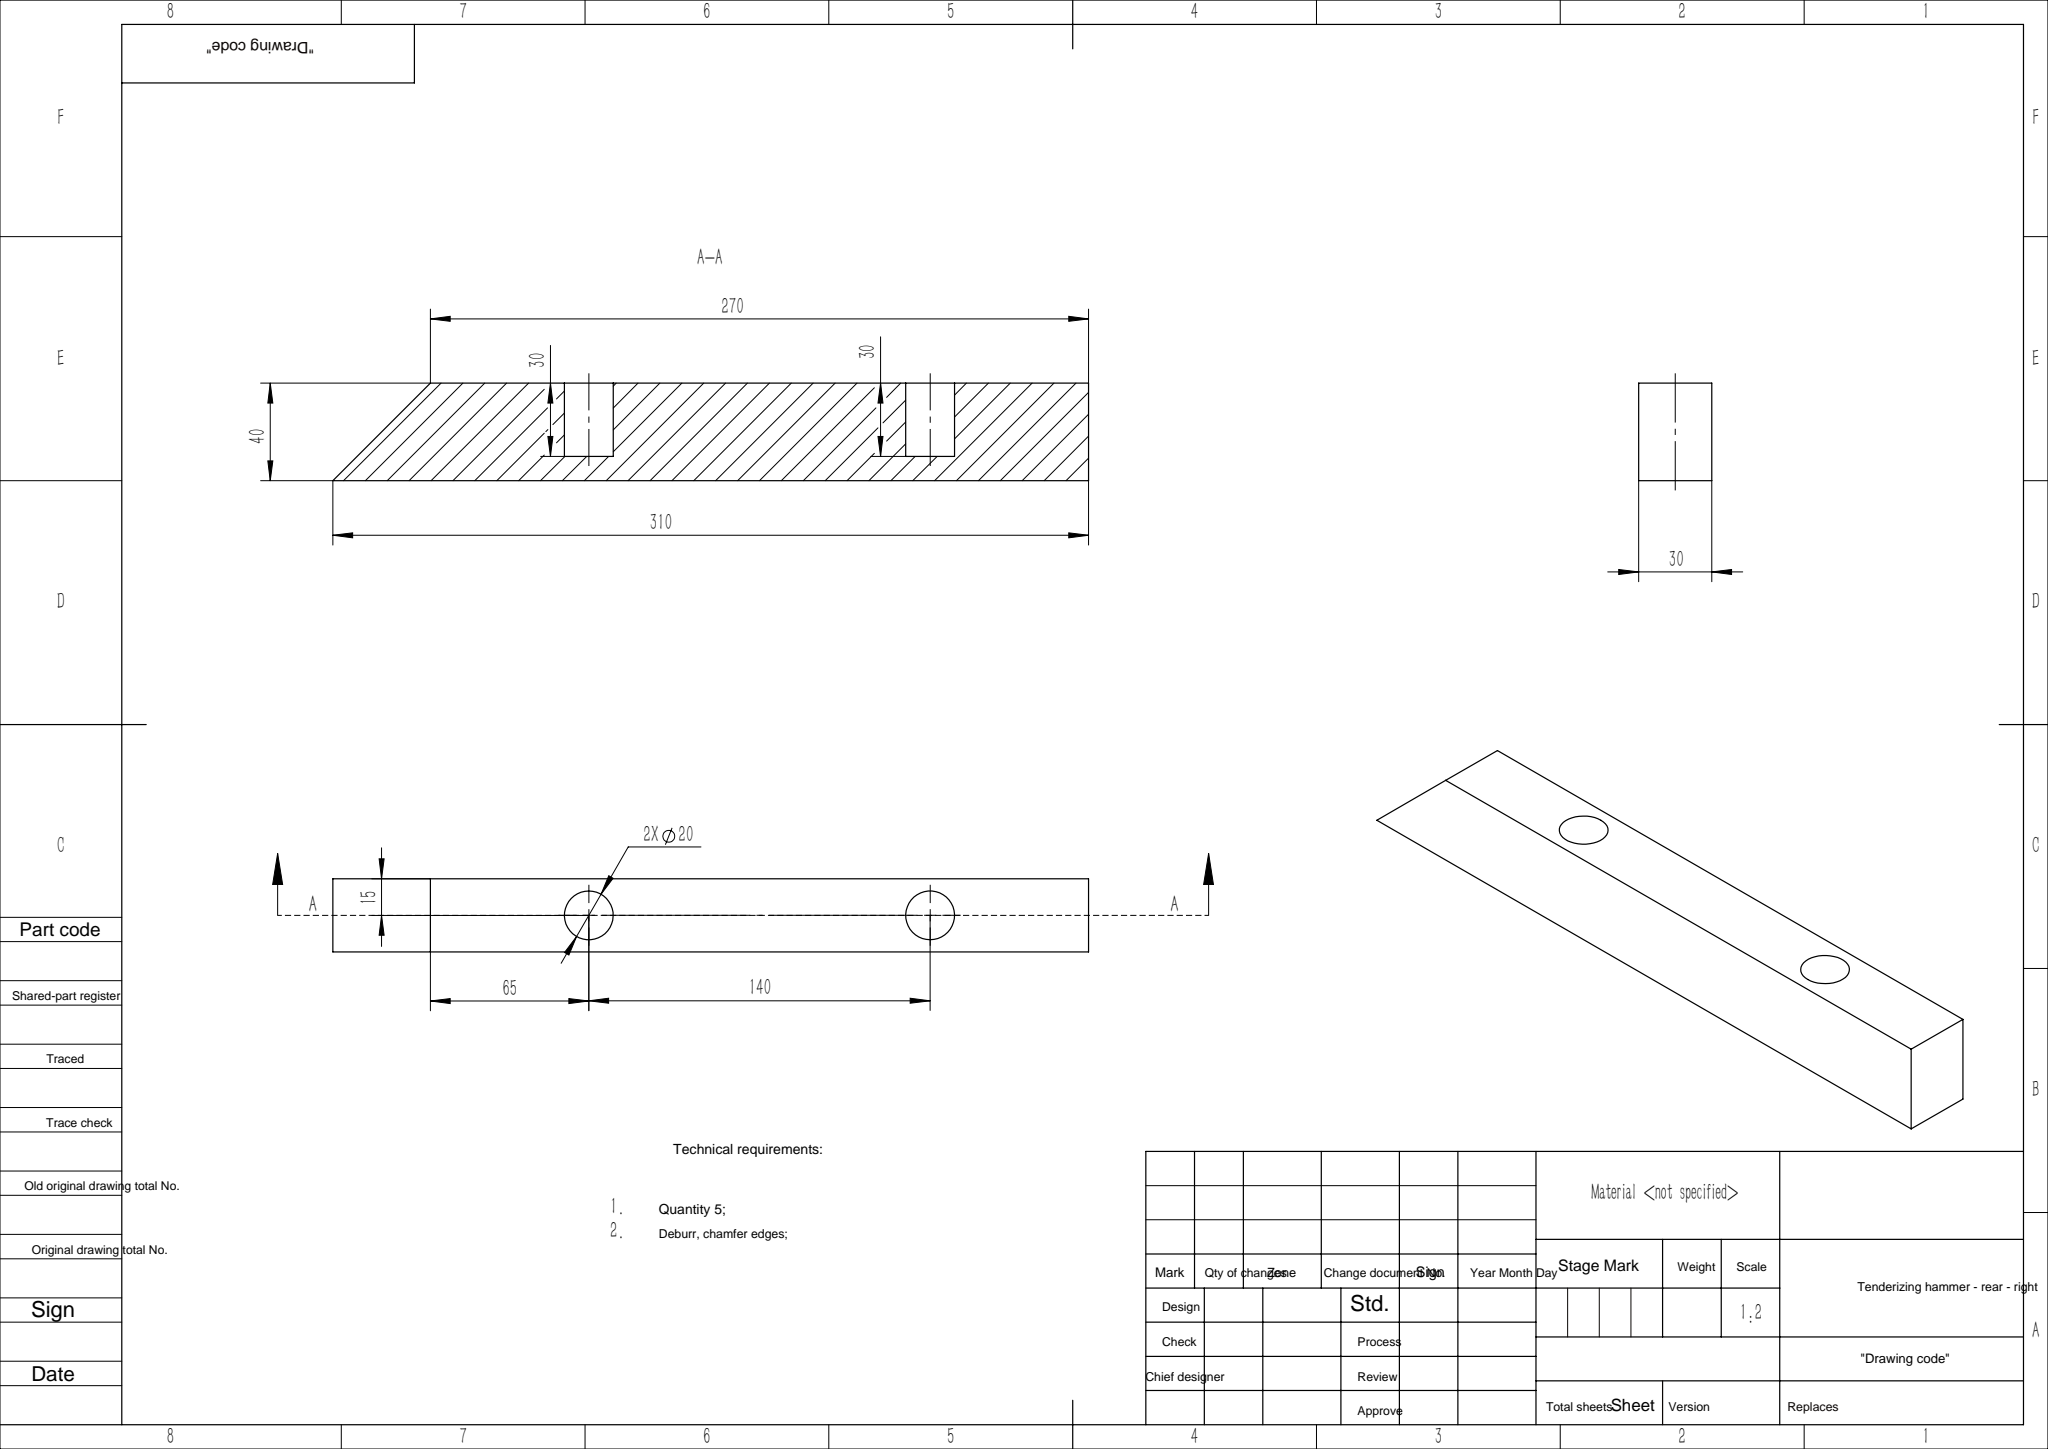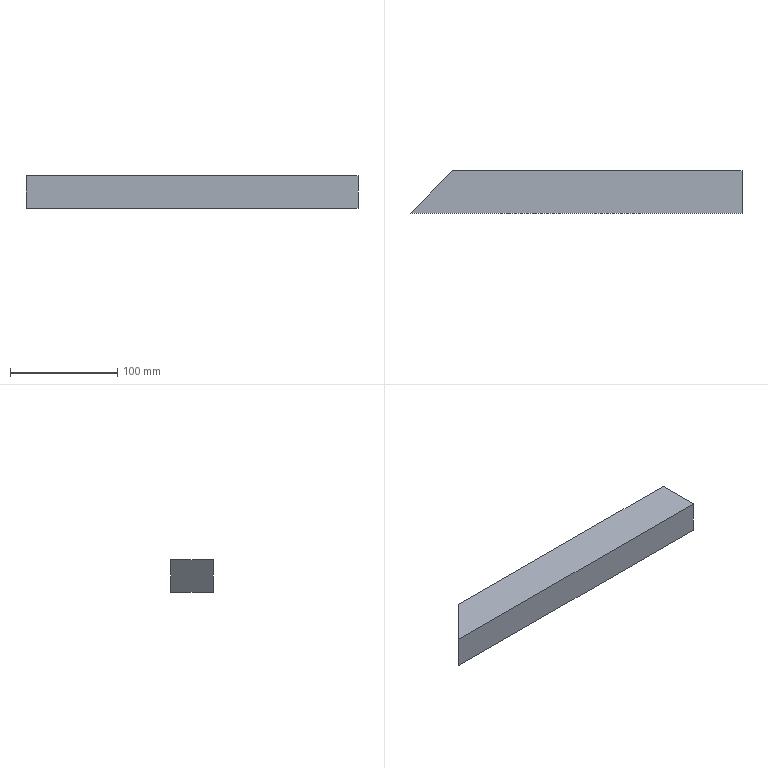Part | SolidWorks | features ICE 3, Extrusion 1 | 1 solid | 12 faces | box 310 x 40 x 30 mm | volume 329150 mm3 | plane 8 | cylinder 4 | commonest cylinder face diameters 20 x4
STEP:
#1=CARTESIAN_POINT('',(-70.,10.,-10.));
#2=VERTEX_POINT('',#1);
#3=CARTESIAN_POINT('',(-70.,10.,10.));
#4=VERTEX_POINT('',#3);
#5=CARTESIAN_POINT('',(-70.,10.,0.));
#6=DIRECTION('',(0.,1.,0.));
#7=DIRECTION('',(0.,0.,-1.));
#8=AXIS2_PLACEMENT_3D('',#5,#6,#7);
#9=CIRCLE('',#8,10.);
#10=EDGE_CURVE('',#2,#4,#9,.T.);
#11=ORIENTED_EDGE('',*,*,#10,.F.);
#12=CARTESIAN_POINT('',(-70.,40.,-10.));
#13=VERTEX_POINT('',#12);
#14=CARTESIAN_POINT('',(-70.,10.,-10.));
#15=DIRECTION('',(0.,1.,0.));
#16=VECTOR('',#15,1000.);
#17=LINE('',#14,#16);
#18=EDGE_CURVE('',#2,#13,#17,.T.);
#19=ORIENTED_EDGE('',*,*,#18,.T.);
#20=CARTESIAN_POINT('',(-70.,40.,10.));
#21=VERTEX_POINT('',#20);
#22=CARTESIAN_POINT('',(-70.,40.,0.));
#23=DIRECTION('',(0.,1.,0.));
#24=DIRECTION('',(0.,0.,-1.));
#25=AXIS2_PLACEMENT_3D('',#22,#23,#24);
#26=CIRCLE('',#25,10.);
#27=EDGE_CURVE('',#13,#21,#26,.T.);
#28=ORIENTED_EDGE('',*,*,#27,.T.);
#29=CARTESIAN_POINT('',(-70.,10.,10.));
#30=DIRECTION('',(0.,1.,0.));
#31=VECTOR('',#30,1000.);
#32=LINE('',#29,#31);
#33=EDGE_CURVE('',#4,#21,#32,.T.);
#34=ORIENTED_EDGE('',*,*,#33,.F.);
#35=EDGE_LOOP('',(#11,#19,#28,#34));
#36=FACE_OUTER_BOUND('',#35,.T.);
#37=CARTESIAN_POINT('',(-70.,10.,0.));
#38=DIRECTION('',(0.,1.,0.));
#39=DIRECTION('',(0.,0.,1.));
#40=AXIS2_PLACEMENT_3D('',#37,#38,#39);
#41=CYLINDRICAL_SURFACE('',#40,10.);
#42=ADVANCED_FACE('',(#36),#41,.F.);
#43=CARTESIAN_POINT('',(70.,10.,-10.));
#44=VERTEX_POINT('',#43);
#45=CARTESIAN_POINT('',(70.,10.,10.));
#46=VERTEX_POINT('',#45);
#47=CARTESIAN_POINT('',(70.,10.,0.));
#48=DIRECTION('',(0.,1.,0.));
#49=DIRECTION('',(0.,0.,1.));
#50=AXIS2_PLACEMENT_3D('',#47,#48,#49);
#51=CIRCLE('',#50,10.);
#52=EDGE_CURVE('',#44,#46,#51,.T.);
#53=ORIENTED_EDGE('',*,*,#52,.F.);
#54=CARTESIAN_POINT('',(70.,40.,-10.));
#55=VERTEX_POINT('',#54);
#56=CARTESIAN_POINT('',(70.,10.,-10.));
#57=DIRECTION('',(0.,1.,0.));
#58=VECTOR('',#57,1000.);
#59=LINE('',#56,#58);
#60=EDGE_CURVE('',#44,#55,#59,.T.);
#61=ORIENTED_EDGE('',*,*,#60,.T.);
#62=CARTESIAN_POINT('',(70.,40.,10.));
#63=VERTEX_POINT('',#62);
#64=CARTESIAN_POINT('',(70.,40.,0.));
#65=DIRECTION('',(0.,1.,0.));
#66=DIRECTION('',(0.,0.,1.));
#67=AXIS2_PLACEMENT_3D('',#64,#65,#66);
#68=CIRCLE('',#67,10.);
#69=EDGE_CURVE('',#55,#63,#68,.T.);
#70=ORIENTED_EDGE('',*,*,#69,.T.);
#71=CARTESIAN_POINT('',(70.,10.,10.));
#72=DIRECTION('',(0.,1.,0.));
#73=VECTOR('',#72,1000.);
#74=LINE('',#71,#73);
#75=EDGE_CURVE('',#46,#63,#74,.T.);
#76=ORIENTED_EDGE('',*,*,#75,.F.);
#77=EDGE_LOOP('',(#53,#61,#70,#76));
#78=FACE_OUTER_BOUND('',#77,.T.);
#79=CARTESIAN_POINT('',(70.,10.,0.));
#80=DIRECTION('',(0.,1.,0.));
#81=DIRECTION('',(0.,0.,1.));
#82=AXIS2_PLACEMENT_3D('',#79,#80,#81);
#83=CYLINDRICAL_SURFACE('',#82,10.);
#84=ADVANCED_FACE('',(#78),#83,.F.);
#85=CARTESIAN_POINT('',(135.,0.,15.));
#86=VERTEX_POINT('',#85);
#87=CARTESIAN_POINT('',(135.,0.,-15.));
#88=VERTEX_POINT('',#87);
#89=CARTESIAN_POINT('',(135.,0.,15.));
#90=DIRECTION('',(0.,0.,-1.));
#91=VECTOR('',#90,1000.);
#92=LINE('',#89,#91);
#93=EDGE_CURVE('',#86,#88,#92,.T.);
#94=ORIENTED_EDGE('',*,*,#93,.T.);
#95=CARTESIAN_POINT('',(135.,40.,-15.));
#96=VERTEX_POINT('',#95);
#97=CARTESIAN_POINT('',(135.,40.,-15.));
#98=DIRECTION('',(0.,-1.,0.));
#99=VECTOR('',#98,1000.);
#100=LINE('',#97,#99);
#101=EDGE_CURVE('',#96,#88,#100,.T.);
#102=ORIENTED_EDGE('',*,*,#101,.F.);
#103=CARTESIAN_POINT('',(135.,40.,15.));
#104=VERTEX_POINT('',#103);
#105=CARTESIAN_POINT('',(135.,40.,15.));
#106=DIRECTION('',(0.,0.,-1.));
#107=VECTOR('',#106,1000.);
#108=LINE('',#105,#107);
#109=EDGE_CURVE('',#104,#96,#108,.T.);
#110=ORIENTED_EDGE('',*,*,#109,.F.);
#111=CARTESIAN_POINT('',(135.,40.,15.));
#112=DIRECTION('',(0.,-1.,0.));
#113=VECTOR('',#112,1000.);
#114=LINE('',#111,#113);
#115=EDGE_CURVE('',#104,#86,#114,.T.);
#116=ORIENTED_EDGE('',*,*,#115,.T.);
#117=EDGE_LOOP('',(#94,#102,#110,#116));
#118=FACE_OUTER_BOUND('',#117,.T.);
#119=CARTESIAN_POINT('',(135.,40.,15.));
#120=DIRECTION('',(-1.,0.,0.));
#121=DIRECTION('',(0.,0.,1.));
#122=AXIS2_PLACEMENT_3D('',#119,#120,#121);
#123=PLANE('',#122);
#124=ADVANCED_FACE('',(#118),#123,.F.);
#125=CARTESIAN_POINT('',(-175.,0.,-15.));
#126=VERTEX_POINT('',#125);
#127=CARTESIAN_POINT('',(-135.,0.,-15.));
#128=DIRECTION('',(-1.,0.,0.));
#129=VECTOR('',#128,1000.);
#130=LINE('',#127,#129);
#131=EDGE_CURVE('',#88,#126,#130,.T.);
#132=ORIENTED_EDGE('',*,*,#131,.T.);
#133=CARTESIAN_POINT('',(-135.,40.,-15.));
#134=VERTEX_POINT('',#133);
#135=CARTESIAN_POINT('',(-175.,0.,-15.));
#136=DIRECTION('',(0.7071,0.7071,0.));
#137=VECTOR('',#136,1000.);
#138=LINE('',#135,#137);
#139=EDGE_CURVE('',#126,#134,#138,.T.);
#140=ORIENTED_EDGE('',*,*,#139,.T.);
#141=CARTESIAN_POINT('',(-135.,40.,-15.));
#142=DIRECTION('',(-1.,0.,0.));
#143=VECTOR('',#142,1000.);
#144=LINE('',#141,#143);
#145=EDGE_CURVE('',#96,#134,#144,.T.);
#146=ORIENTED_EDGE('',*,*,#145,.F.);
#147=ORIENTED_EDGE('',*,*,#101,.T.);
#148=EDGE_LOOP('',(#132,#140,#146,#147));
#149=FACE_OUTER_BOUND('',#148,.T.);
#150=CARTESIAN_POINT('',(-135.,40.,-15.));
#151=DIRECTION('',(0.,0.,1.));
#152=DIRECTION('',(1.,0.,0.));
#153=AXIS2_PLACEMENT_3D('',#150,#151,#152);
#154=PLANE('',#153);
#155=ADVANCED_FACE('',(#149),#154,.F.);
#156=CARTESIAN_POINT('',(-135.,40.,15.));
#157=VERTEX_POINT('',#156);
#158=CARTESIAN_POINT('',(-135.,40.,15.));
#159=DIRECTION('',(1.,0.,0.));
#160=VECTOR('',#159,1000.);
#161=LINE('',#158,#160);
#162=EDGE_CURVE('',#157,#104,#161,.T.);
#163=ORIENTED_EDGE('',*,*,#162,.F.);
#164=CARTESIAN_POINT('',(-175.,0.,15.));
#165=VERTEX_POINT('',#164);
#166=CARTESIAN_POINT('',(-175.,0.,15.));
#167=DIRECTION('',(0.7071,0.7071,0.));
#168=VECTOR('',#167,1000.);
#169=LINE('',#166,#168);
#170=EDGE_CURVE('',#165,#157,#169,.T.);
#171=ORIENTED_EDGE('',*,*,#170,.F.);
#172=CARTESIAN_POINT('',(-135.,0.,15.));
#173=DIRECTION('',(1.,0.,0.));
#174=VECTOR('',#173,1000.);
#175=LINE('',#172,#174);
#176=EDGE_CURVE('',#165,#86,#175,.T.);
#177=ORIENTED_EDGE('',*,*,#176,.T.);
#178=ORIENTED_EDGE('',*,*,#115,.F.);
#179=EDGE_LOOP('',(#163,#171,#177,#178));
#180=FACE_OUTER_BOUND('',#179,.T.);
#181=CARTESIAN_POINT('',(-135.,40.,15.));
#182=DIRECTION('',(0.,0.,-1.));
#183=DIRECTION('',(-1.,0.,0.));
#184=AXIS2_PLACEMENT_3D('',#181,#182,#183);
#185=PLANE('',#184);
#186=ADVANCED_FACE('',(#180),#185,.F.);
#187=CARTESIAN_POINT('',(-70.,40.,0.));
#188=DIRECTION('',(0.,1.,0.));
#189=DIRECTION('',(0.,0.,-1.));
#190=AXIS2_PLACEMENT_3D('',#187,#188,#189);
#191=CIRCLE('',#190,10.);
#192=EDGE_CURVE('',#21,#13,#191,.T.);
#193=ORIENTED_EDGE('',*,*,#192,.F.);
#194=ORIENTED_EDGE('',*,*,#27,.F.);
#195=EDGE_LOOP('',(#193,#194));
#196=FACE_BOUND('',#195,.T.);
#197=CARTESIAN_POINT('',(70.,40.,0.));
#198=DIRECTION('',(0.,1.,0.));
#199=DIRECTION('',(0.,0.,1.));
#200=AXIS2_PLACEMENT_3D('',#197,#198,#199);
#201=CIRCLE('',#200,10.);
#202=EDGE_CURVE('',#63,#55,#201,.T.);
#203=ORIENTED_EDGE('',*,*,#202,.F.);
#204=ORIENTED_EDGE('',*,*,#69,.F.);
#205=EDGE_LOOP('',(#203,#204));
#206=FACE_BOUND('',#205,.T.);
#207=ORIENTED_EDGE('',*,*,#145,.T.);
#208=CARTESIAN_POINT('',(-135.,40.,-15.));
#209=DIRECTION('',(0.,0.,1.));
#210=VECTOR('',#209,1000.);
#211=LINE('',#208,#210);
#212=EDGE_CURVE('',#134,#157,#211,.T.);
#213=ORIENTED_EDGE('',*,*,#212,.T.);
#214=ORIENTED_EDGE('',*,*,#162,.T.);
#215=ORIENTED_EDGE('',*,*,#109,.T.);
#216=EDGE_LOOP('',(#207,#213,#214,#215));
#217=FACE_OUTER_BOUND('',#216,.T.);
#218=CARTESIAN_POINT('',(0.,40.,0.));
#219=DIRECTION('',(0.,-1.,0.));
#220=DIRECTION('',(0.,0.,-1.));
#221=AXIS2_PLACEMENT_3D('',#218,#219,#220);
#222=PLANE('',#221);
#223=ADVANCED_FACE('',(#196,#206,#217),#222,.F.);
#224=ORIENTED_EDGE('',*,*,#93,.F.);
#225=ORIENTED_EDGE('',*,*,#176,.F.);
#226=CARTESIAN_POINT('',(-175.,0.,-15.));
#227=DIRECTION('',(0.,0.,1.));
#228=VECTOR('',#227,1000.);
#229=LINE('',#226,#228);
#230=EDGE_CURVE('',#126,#165,#229,.T.);
#231=ORIENTED_EDGE('',*,*,#230,.F.);
#232=ORIENTED_EDGE('',*,*,#131,.F.);
#233=EDGE_LOOP('',(#224,#225,#231,#232));
#234=FACE_OUTER_BOUND('',#233,.T.);
#235=CARTESIAN_POINT('',(0.,0.,0.));
#236=DIRECTION('',(0.,-1.,0.));
#237=DIRECTION('',(0.,0.,-1.));
#238=AXIS2_PLACEMENT_3D('',#235,#236,#237);
#239=PLANE('',#238);
#240=ADVANCED_FACE('',(#234),#239,.T.);
#241=ORIENTED_EDGE('',*,*,#60,.F.);
#242=CARTESIAN_POINT('',(70.,10.,0.));
#243=DIRECTION('',(0.,1.,0.));
#244=DIRECTION('',(0.,0.,1.));
#245=AXIS2_PLACEMENT_3D('',#242,#243,#244);
#246=CIRCLE('',#245,10.);
#247=EDGE_CURVE('',#46,#44,#246,.T.);
#248=ORIENTED_EDGE('',*,*,#247,.F.);
#249=ORIENTED_EDGE('',*,*,#75,.T.);
#250=ORIENTED_EDGE('',*,*,#202,.T.);
#251=EDGE_LOOP('',(#241,#248,#249,#250));
#252=FACE_OUTER_BOUND('',#251,.T.);
#253=CARTESIAN_POINT('',(70.,10.,0.));
#254=DIRECTION('',(0.,1.,0.));
#255=DIRECTION('',(0.,0.,1.));
#256=AXIS2_PLACEMENT_3D('',#253,#254,#255);
#257=CYLINDRICAL_SURFACE('',#256,10.);
#258=ADVANCED_FACE('',(#252),#257,.F.);
#259=ORIENTED_EDGE('',*,*,#247,.T.);
#260=ORIENTED_EDGE('',*,*,#52,.T.);
#261=EDGE_LOOP('',(#259,#260));
#262=FACE_OUTER_BOUND('',#261,.T.);
#263=CARTESIAN_POINT('',(70.,10.,0.));
#264=DIRECTION('',(0.,1.,0.));
#265=DIRECTION('',(0.,0.,1.));
#266=AXIS2_PLACEMENT_3D('',#263,#264,#265);
#267=PLANE('',#266);
#268=ADVANCED_FACE('',(#262),#267,.T.);
#269=ORIENTED_EDGE('',*,*,#18,.F.);
#270=CARTESIAN_POINT('',(-70.,10.,0.));
#271=DIRECTION('',(0.,1.,0.));
#272=DIRECTION('',(0.,0.,-1.));
#273=AXIS2_PLACEMENT_3D('',#270,#271,#272);
#274=CIRCLE('',#273,10.);
#275=EDGE_CURVE('',#4,#2,#274,.T.);
#276=ORIENTED_EDGE('',*,*,#275,.F.);
#277=ORIENTED_EDGE('',*,*,#33,.T.);
#278=ORIENTED_EDGE('',*,*,#192,.T.);
#279=EDGE_LOOP('',(#269,#276,#277,#278));
#280=FACE_OUTER_BOUND('',#279,.T.);
#281=CARTESIAN_POINT('',(-70.,10.,0.));
#282=DIRECTION('',(0.,1.,0.));
#283=DIRECTION('',(0.,0.,1.));
#284=AXIS2_PLACEMENT_3D('',#281,#282,#283);
#285=CYLINDRICAL_SURFACE('',#284,10.);
#286=ADVANCED_FACE('',(#280),#285,.F.);
#287=ORIENTED_EDGE('',*,*,#275,.T.);
#288=ORIENTED_EDGE('',*,*,#10,.T.);
#289=EDGE_LOOP('',(#287,#288));
#290=FACE_OUTER_BOUND('',#289,.T.);
#291=CARTESIAN_POINT('',(-70.,10.,0.));
#292=DIRECTION('',(0.,-1.,0.));
#293=DIRECTION('',(0.,0.,-1.));
#294=AXIS2_PLACEMENT_3D('',#291,#292,#293);
#295=PLANE('',#294);
#296=ADVANCED_FACE('',(#290),#295,.F.);
#297=ORIENTED_EDGE('',*,*,#170,.T.);
#298=ORIENTED_EDGE('',*,*,#212,.F.);
#299=ORIENTED_EDGE('',*,*,#139,.F.);
#300=ORIENTED_EDGE('',*,*,#230,.T.);
#301=EDGE_LOOP('',(#297,#298,#299,#300));
#302=FACE_OUTER_BOUND('',#301,.T.);
#303=CARTESIAN_POINT('',(-175.,0.,-15.));
#304=DIRECTION('',(0.7071,-0.7071,0.));
#305=DIRECTION('',(0.7071,0.7071,0.));
#306=AXIS2_PLACEMENT_3D('',#303,#304,#305);
#307=PLANE('',#306);
#308=ADVANCED_FACE('',(#302),#307,.F.);
#309=CLOSED_SHELL('',(#42,#84,#124,#155,#186,#223,#240,#258,#268,#286,#296,#308));
#310=MANIFOLD_SOLID_BREP('',#309);
#311=CARTESIAN_POINT('',(0.,0.,0.));
#312=DIRECTION('',(0.,0.,1.));
#313=DIRECTION('',(1.,0.,0.));
#314=AXIS2_PLACEMENT_3D('',#311,#312,#313);
#315=(LENGTH_UNIT()NAMED_UNIT(*)SI_UNIT(.MILLI.,.METRE.));
#316=UNCERTAINTY_MEASURE_WITH_UNIT(LENGTH_MEASURE(0.00001),#315,'','');
#317=(NAMED_UNIT(*)PLANE_ANGLE_UNIT()SI_UNIT($,.RADIAN.));
#318=(NAMED_UNIT(*)SI_UNIT($,.STERADIAN.)SOLID_ANGLE_UNIT());
#319=(GEOMETRIC_REPRESENTATION_CONTEXT(3)GLOBAL_UNCERTAINTY_ASSIGNED_CONTEXT((#316))GLOBAL_UNIT_ASSIGNED_CONTEXT((#315,#317,#318))REPRESENTATION_CONTEXT('',''));
#320=ADVANCED_BREP_SHAPE_REPRESENTATION('',(#310,#314),#319);